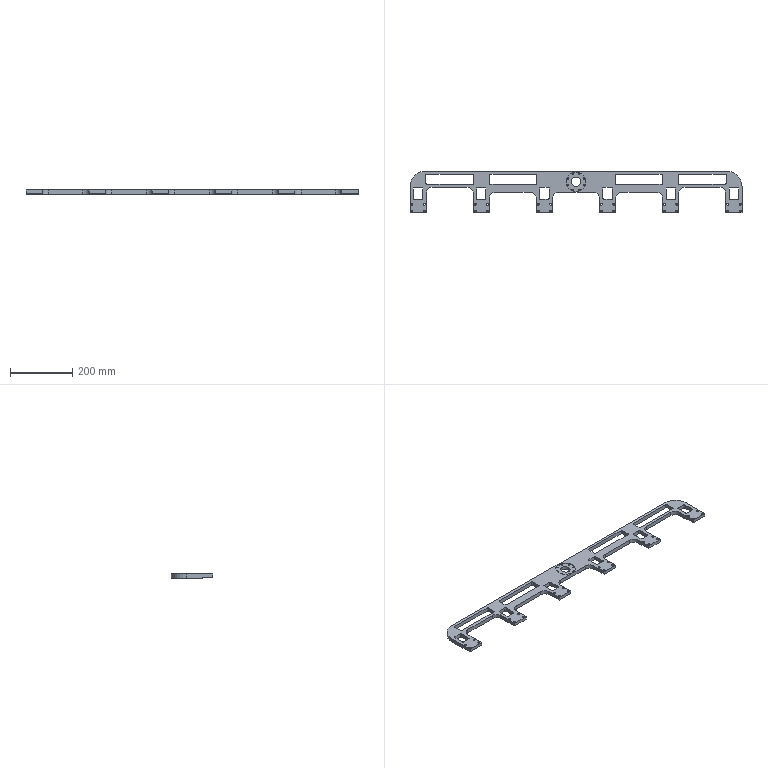NC program | NX | posted with a generic post | part box 1068 x 134 x 13 mm
Lines 9073 to 9724 of 9724:
(PLANAR_MILL_COPY_1 , TOOL : D6A45)
N18084 T07 M6
N18086 G54
N18088 G17 G0 G90 X128.785 Y-35.086 S9500 M3
N18090 G43 Z30. H7
N18092 Z0.
N18094 G94 G1 Z-1. F1400.
N18096 X128.512 Y-34.706
N18098 G3 X127.6 Y-34.295 R1.
N18100 G1 X127.5 Y-34.3
N18102 X75.7
N18104 G2 X74.7 Y-33.3 R1.
N18106 G1 Y-20.95
N18108 G3 X55.6 Y-1.85 R19.1
N18110 G1 X-55.6
N18112 G3 X-74.7 Y-20.95 R19.1
N18114 G1 Y-33.3
N18116 G2 X-75.7 Y-34.3 R1.
N18118 G1 X-127.5
N18120 G2 X-128.5 Y-33.3 R1.
N18122 G1 Y-20.95
N18124 G3 X-147.6 Y-1.85 R19.1
N18126 G1 X-258.8
N18128 G3 X-277.9 Y-20.95 R19.1
N18130 G1 Y-33.3
N18132 G2 X-278.9 Y-34.3 R1.
N18134 G1 X-330.7
N18136 G2 X-331.7 Y-33.3 R1.
N18138 G1 Y-5.
N18140 G3 X-350.8 Y14.1 R19.1
N18142 G1 X-462.
N18144 G3 X-481.1 Y-5. R19.1
N18146 G1 Y-33.3
N18148 G2 X-482.1 Y-34.3 R1.
N18150 G1 X-533.9
N18152 G2 X-534.9 Y-33.3 R1.
N18154 G1 Y17.
N18156 G2 X-484. Y67.9 R50.9
N18158 G1 X127.6
N18160 G3 X128.466 Y68.4 R1.
N18162 G1 X128.87 Y69.1
N18164 Z0.
N18166 G0 Z30.
N18168 X88.7 Y-2.73
N18170 Z0.
N18172 G1 Z-1.
N18174 X88. Y-3.134
N18176 G3 X87.5 Y-4. R1.
N18178 G1 Y-21.
N18180 G3 X89.6 Y-23.1 R2.1
N18182 G1 X113.6
N18184 G3 X115.7 Y-21. R2.1
N18186 G1 Y13.
N18188 G3 X113.6 Y15.1 R2.1
N18190 G1 X89.6
N18192 G3 X87.5 Y13. R2.1
N18194 G1 Y-4.
N18196 G3 X88. Y-4.866 R1.
N18198 G1 X88.7 Y-5.27
N18200 Z0.
N18202 G0 Z30.
N18204 X128.977 Y54.649
N18206 Z0.
N18208 G1 Z-1.
N18210 X128.34 Y55.313
N18212 G3 X127.6 Y54.64 R1.
N18214 X127.5 Y54. R2.1
N18216 G1 Y28.
N18218 G3 X127.6 Y27.36 R2.1
N18220 X128.34 Y26.687 R1.
N18222 G1 X128.977 Y27.351
N18224 Z0.
N18226 G0 Z30.
N18228 X26.469 Y45.518
N18230 Z0.
N18232 G1 Z-1.
N18234 X26.735 Y46.315
N18236 G3 X25.869 Y46.815 R1.
N18238 X22.769 Y43.715 R3.1
N18240 X25.869 Y46.815 R-3.1
N18242 X25.003 Y46.315 R1.
N18244 G1 X25.268 Y45.518
N18246 Z0.
N18248 G0 Z30.
N18250 X11.316 Y60.671
N18252 Z0.
N18254 G1 Z-1.
N18256 X11.581 Y61.469
N18258 G3 X10.715 Y61.969 R1.
N18260 X7.615 Y58.869 R3.1
N18262 X10.715 Y61.969 R-3.1
N18264 X9.849 Y61.469 R1.
N18266 G1 X10.115 Y60.671
N18268 Z0.
N18270 G0 Z30.
N18272 X-10.115
N18274 Z0.
N18276 G1 Z-1.
N18278 X-9.849 Y61.469
N18280 G3 X-10.715 Y61.969 R1.
N18282 X-13.815 Y58.869 R3.1
N18284 X-10.715 Y61.969 R-3.1
N18286 X-11.581 Y61.469 R1.
N18288 G1 X-11.316 Y60.671
N18290 Z0.
N18292 G0 Z30.
N18294 X-25.268 Y45.518
N18296 Z0.
N18298 G1 Z-1.
N18300 X-25.003 Y46.315
N18302 G3 X-25.869 Y46.815 R1.
N18304 X-28.969 Y43.715 R3.1
N18306 X-25.869 Y46.815 R-3.1
N18308 X-26.735 Y46.315 R1.
N18310 G1 X-26.469 Y45.518
N18312 Z0.
N18314 G0 Z30.
N18316 X1.309 Y45.833
N18318 Z0.
N18320 G1 Z-1.
N18322 X0.866 Y46.6
N18324 G3 X0. Y47.1 R1.
N18326 X-14.1 Y33. R14.1
N18328 X0. Y47.1 R-14.1
N18330 X-0.866 Y46.6 R1.
N18332 G1 X-1.309 Y45.833
N18334 Z0.
N18336 G0 Z30.
N18338 X26.469 Y24.087
N18340 Z0.
N18342 G1 Z-1.
N18344 X26.735 Y24.885
N18346 G3 X25.869 Y25.385 R1.
N18348 X22.769 Y22.285 R3.1
N18350 X25.869 Y25.385 R-3.1
N18352 X25.003 Y24.885 R1.
N18354 G1 X25.268 Y24.087
N18356 Z0.
N18358 G0 Z30.
N18360 X10.115 Y5.329
N18362 Z0.
N18364 G1 Z-1.
N18366 X9.849 Y4.531
N18368 G3 X10.715 Y4.031 R1.
N18370 X13.815 Y7.131 R3.1
N18372 X10.715 Y4.031 R-3.1
N18374 X11.581 Y4.531 R1.
N18376 G1 X11.316 Y5.329
N18378 Z0.
N18380 G0 Z30.
N18382 X-11.316
N18384 Z0.
N18386 G1 Z-1.
N18388 X-11.581 Y4.531
N18390 G3 X-10.715 Y4.031 R1.
N18392 X-7.615 Y7.131 R3.1
N18394 X-10.715 Y4.031 R-3.1
N18396 X-9.849 Y4.531 R1.
N18398 G1 X-10.115 Y5.329
N18400 Z0.
N18402 G0 Z30.
N18404 X-25.268 Y24.087
N18406 Z0.
N18408 G1 Z-1.
N18410 X-25.003 Y24.885
N18412 G3 X-25.869 Y25.385 R1.
N18414 X-28.969 Y22.285 R3.1
N18416 X-25.869 Y25.385 R-3.1
N18418 X-26.735 Y24.885 R1.
N18420 G1 X-26.469 Y24.087
N18422 Z0.
N18424 G0 Z30.
N18426 X-88.7 Y-5.27
N18428 Z0.
N18430 G1 Z-1.
N18432 X-88. Y-4.866
N18434 G3 X-87.5 Y-4. R1.
N18436 G1 Y13.
N18438 G3 X-89.6 Y15.1 R2.1
N18440 G1 X-113.6
N18442 G3 X-115.7 Y13. R2.1
N18444 G1 Y-21.
N18446 G3 X-113.6 Y-23.1 R2.1
N18448 G1 X-89.6
N18450 G3 X-87.5 Y-21. R2.1
N18452 G1 Y-4.
N18454 G3 X-88. Y-3.134 R1.
N18456 G1 X-88.7 Y-2.73
N18458 Z0.
N18460 G0 Z30.
N18462 X-201.93 Y54.9
N18464 Z0.
N18466 G1 Z-1.
N18468 X-202.334 Y55.6
N18470 G3 X-203.2 Y56.1 R1.
N18472 G1 X-276.8
N18474 G3 X-278.9 Y54. R2.1
N18476 G1 Y28.
N18478 G3 X-276.8 Y25.9 R2.1
N18480 G1 X-129.6
N18482 G3 X-127.5 Y28. R2.1
N18484 G1 Y54.
N18486 G3 X-129.6 Y56.1 R2.1
N18488 G1 X-203.2
N18490 G3 X-204.066 Y55.6 R1.
N18492 G1 X-204.47 Y54.9
N18494 Z0.
N18496 G0 Z30.
N18498 X-291.9 Y-5.27
N18500 Z0.
N18502 G1 Z-1.
N18504 X-291.2 Y-4.866
N18506 G3 X-290.7 Y-4. R1.
N18508 G1 Y13.
N18510 G3 X-292.8 Y15.1 R2.1
N18512 G1 X-316.8
N18514 G3 X-318.9 Y13. R2.1
N18516 G1 Y-21.
N18518 G3 X-316.8 Y-23.1 R2.1
N18520 G1 X-292.8
N18522 G3 X-290.7 Y-21. R2.1
N18524 G1 Y-4.
N18526 G3 X-291.2 Y-3.134 R1.
N18528 G1 X-291.9 Y-2.73
N18530 Z0.
N18532 G0 Z30.
N18534 X-405.13 Y54.9
N18536 Z0.
N18538 G1 Z-1.
N18540 X-405.534 Y55.6
N18542 G3 X-406.4 Y56.1 R1.
N18544 G1 X-480.
N18546 G3 X-482.1 Y54. R2.1
N18548 G1 Y28.
N18550 G3 X-480. Y25.9 R2.1
N18552 G1 X-332.8
N18554 G3 X-330.7 Y28. R2.1
N18556 G1 Y54.
N18558 G3 X-332.8 Y56.1 R2.1
N18560 G1 X-406.4
N18562 G3 X-407.266 Y55.6 R1.
N18564 G1 X-407.67 Y54.9
N18566 Z0.
N18568 G0 Z30.
N18570 X-520.9 Y-2.73
N18572 Z0.
N18574 G1 Z-1.
N18576 X-521.6 Y-3.134
N18578 G3 X-522.1 Y-4. R1.
N18580 G1 Y-21.
N18582 G3 X-520. Y-23.1 R2.1
N18584 G1 X-496.
N18586 G3 X-493.9 Y-21. R2.1
N18588 G1 Y13.
N18590 G3 X-496. Y15.1 R2.1
N18592 G1 X-520.
N18594 G3 X-522.1 Y13. R2.1
N18596 G1 Y-4.
N18598 G3 X-521.6 Y-4.866 R1.
N18600 G1 X-520.9 Y-5.27
N18602 Z0.
N18604 G0 Z30.
(PLANAR_MILL_COPY_COPY , TOOL : D6A45)
N18606 X121.593 Y-38.1
N18608 Z-3.
N18610 G1 Z-4.
N18612 Y-37.056
N18614 G3 X121.118 Y-36.9 R0.5
N18616 X122.082 Y-36.9 R-2.35
N18618 X121.607 Y-37.056 R0.5
N18620 G1 Y-38.1
N18622 Z-3.
N18624 G0 Z30.
N18626 X121.112 Y-62.242
N18628 Z-3.
N18630 G1 Z-4.
N18632 X120.734 Y-63.05
N18634 G3 X121.6 Y-63.55 R1.
N18636 X123.95 Y-61.2 R2.35
N18638 X121.6 Y-63.55 R-2.35
N18640 X122.466 Y-63.05 R1.
N18642 G1 X122.088 Y-62.242
N18644 Z-3.
N18646 G0 Z30.
N18648 X129.913 Y-37.492
N18650 Z-3.
N18652 G1 Z-4.
N18654 X129.465 Y-37.043
N18656 G3 X128.5 Y-36.782 R1.
N18658 G1 Y-66.9
N18660 G2 X127.5 Y-67.9 R1.
N18662 G1 X75.7
N18664 G2 X74.7 Y-66.9 R1.
N18666 G1 Y-36.782
N18668 G3 X73.735 Y-37.043 R1.
N18670 G1 X73.287 Y-37.492
N18672 Z-3.
N18674 G0 Z30.
N18676 X-73.287
N18678 Z-3.
N18680 G1 Z-4.
N18682 X-73.735 Y-37.043
N18684 G3 X-74.7 Y-36.782 R1.
N18686 G1 Y-66.9
N18688 G2 X-75.7 Y-67.9 R1.
N18690 G1 X-127.5
N18692 G2 X-128.5 Y-66.9 R1.
N18694 G1 Y-36.782
N18696 G3 X-129.465 Y-37.043 R1.
N18698 G1 X-129.913 Y-37.492
N18700 Z-3.
N18702 G0 Z30.
N18704 X-276.487
N18706 Z-3.
N18708 G1 Z-4.
N18710 X-276.935 Y-37.043
N18712 G3 X-277.9 Y-36.782 R1.
N18714 G1 Y-66.9
N18716 G2 X-278.9 Y-67.9 R1.
N18718 G1 X-330.7
N18720 G2 X-331.7 Y-66.9 R1.
N18722 G1 Y-36.782
N18724 G3 X-332.665 Y-37.043 R1.
N18726 G1 X-333.113 Y-37.492
N18728 Z-3.
N18730 G0 Z30.
N18732 X-479.687
N18734 Z-3.
N18736 G1 Z-4.
N18738 X-480.135 Y-37.043
N18740 G3 X-481.1 Y-36.782 R1.
N18742 G1 Y-66.9
N18744 G2 X-482.1 Y-67.9 R1.
N18746 G1 X-533.9
N18748 G2 X-534.9 Y-66.9 R1.
N18750 G1 Y-36.782
N18752 G3 X-535.865 Y-37.043 R1.
N18754 G1 X-536.313 Y-37.492
N18756 Z-3.
N18758 G0 Z30.
N18760 X81.112 Y-62.242
N18762 Z-3.
N18764 G1 Z-4.
N18766 X80.734 Y-63.05
N18768 G3 X81.6 Y-63.55 R1.
N18770 X83.95 Y-61.2 R2.35
N18772 X81.6 Y-63.55 R-2.35
N18774 X82.466 Y-63.05 R1.
N18776 G1 X82.088 Y-62.242
N18778 Z-3.
N18780 G0 Z30.
N18782 X81.593 Y-38.1
N18784 Z-3.
N18786 G1 Z-4.
N18788 Y-37.056
N18790 G3 X81.118 Y-36.9 R0.5
N18792 X82.082 Y-36.9 R-2.35
N18794 X81.607 Y-37.056 R0.5
N18796 G1 Y-38.1
N18798 Z-3.
N18800 G0 Z30.
N18802 X-81.607
N18804 Z-3.
N18806 G1 Z-4.
N18808 Y-37.056
N18810 G3 X-82.082 Y-36.9 R0.5
N18812 X-81.118 Y-36.9 R-2.35
N18814 X-81.593 Y-37.056 R0.5
N18816 G1 Y-38.1
N18818 Z-3.
N18820 G0 Z30.
N18822 X-82.088 Y-62.242
N18824 Z-3.
N18826 G1 Z-4.
N18828 X-82.466 Y-63.05
N18830 G3 X-81.6 Y-63.55 R1.
N18832 X-79.25 Y-61.2 R2.35
N18834 X-81.6 Y-63.55 R-2.35
N18836 X-80.734 Y-63.05 R1.
N18838 G1 X-81.112 Y-62.242
N18840 Z-3.
N18842 G0 Z30.
N18844 X-122.088
N18846 Z-3.
N18848 G1 Z-4.
N18850 X-122.466 Y-63.05
N18852 G3 X-121.6 Y-63.55 R1.
N18854 X-119.25 Y-61.2 R2.35
N18856 X-121.6 Y-63.55 R-2.35
N18858 X-120.734 Y-63.05 R1.
N18860 G1 X-121.112 Y-62.242
N18862 Z-3.
N18864 G0 Z30.
N18866 X-121.607 Y-38.1
N18868 Z-3.
N18870 G1 Z-4.
N18872 Y-37.056
N18874 G3 X-122.082 Y-36.9 R0.5
N18876 X-121.118 Y-36.9 R-2.35
N18878 X-121.593 Y-37.056 R0.5
N18880 G1 Y-38.1
N18882 Z-3.
N18884 G0 Z30.
N18886 X-284.807
N18888 Z-3.
N18890 G1 Z-4.
N18892 Y-37.056
N18894 G3 X-285.282 Y-36.9 R0.5
N18896 X-284.318 Y-36.9 R-2.35
N18898 X-284.793 Y-37.056 R0.5
N18900 G1 Y-38.1
N18902 Z-3.
N18904 G0 Z30.
N18906 X-285.288 Y-62.242
N18908 Z-3.
N18910 G1 Z-4.
N18912 X-285.666 Y-63.05
N18914 G3 X-284.8 Y-63.55 R1.
N18916 X-282.45 Y-61.2 R2.35
N18918 X-284.8 Y-63.55 R-2.35
N18920 X-283.934 Y-63.05 R1.
N18922 G1 X-284.312 Y-62.242
N18924 Z-3.
N18926 G0 Z30.
N18928 X-325.288
N18930 Z-3.
N18932 G1 Z-4.
N18934 X-325.666 Y-63.05
N18936 G3 X-324.8 Y-63.55 R1.
N18938 X-322.45 Y-61.2 R2.35
N18940 X-324.8 Y-63.55 R-2.35
N18942 X-323.934 Y-63.05 R1.
N18944 G1 X-324.312 Y-62.242
N18946 Z-3.
N18948 G0 Z30.
N18950 X-324.807 Y-38.1
N18952 Z-3.
N18954 G1 Z-4.
N18956 Y-37.056
N18958 G3 X-325.282 Y-36.9 R0.5
N18960 X-324.318 Y-36.9 R-2.35
N18962 X-324.793 Y-37.056 R0.5
N18964 G1 Y-38.1
N18966 Z-3.
N18968 G0 Z30.
N18970 X-488.007
N18972 Z-3.
N18974 G1 Z-4.
N18976 Y-37.056
N18978 G3 X-488.482 Y-36.9 R0.5
N18980 X-487.518 Y-36.9 R-2.35
N18982 X-487.993 Y-37.056 R0.5
N18984 G1 Y-38.1
N18986 Z-3.
N18988 G0 Z30.
N18990 X-488.488 Y-62.242
N18992 Z-3.
N18994 G1 Z-4.
N18996 X-488.866 Y-63.05
N18998 G3 X-488. Y-63.55 R1.
N19000 X-485.65 Y-61.2 R2.35
N19002 X-488. Y-63.55 R-2.35
N19004 X-487.134 Y-63.05 R1.
N19006 G1 X-487.512 Y-62.242
N19008 Z-3.
N19010 G0 Z30.
N19012 X-528.488
N19014 Z-3.
N19016 G1 Z-4.
N19018 X-528.866 Y-63.05
N19020 G3 X-528. Y-63.55 R1.
N19022 X-525.65 Y-61.2 R2.35
N19024 X-528. Y-63.55 R-2.35
N19026 X-527.134 Y-63.05 R1.
N19028 G1 X-527.512 Y-62.242
N19030 Z-3.
N19032 G0 Z30.
N19034 X-528.007 Y-38.1
N19036 Z-3.
N19038 G1 Z-4.
N19040 Y-37.056
N19042 G3 X-528.482 Y-36.9 R0.5
N19044 X-527.518 Y-36.9 R-2.35
N19046 X-527.993 Y-37.056 R0.5
N19048 G1 Y-38.1
N19050 Z-3.
N19052 G0 Z30.
N19054 M5
(ZLEVEL_PROFILE_COPY_3_COPY , TOOL : D10)
N19056 T10 M6
N19058 G54
N19060 G17 G0 G90 X129.999 Y-75.155 S9500 M3
N19062 G43 Z30. H10
N19064 Z-7.525
N19066 G94 G1 Z-12.525 F1000.
N19068 X128.466 Y-72.5
N19070 G3 X127.6 Y-72. R1.
N19072 G1 X75.6 F1200.
N19074 G2 X70.6 Y-67. R5.
N19076 G1 Y-20.95
N19078 G3 X55.6 Y-5.95 R15.
N19080 G1 X-55.6
N19082 G3 X-70.6 Y-20.95 R15.
N19084 G1 Y-67.
N19086 G2 X-75.6 Y-72. R5.
N19088 G1 X-127.6
N19090 G2 X-132.6 Y-67. R5.
N19092 G1 Y-20.95
N19094 G3 X-147.6 Y-5.95 R15.
N19096 G1 X-258.8
N19098 G3 X-273.8 Y-20.95 R15.
N19100 G1 Y-67.
N19102 G2 X-278.8 Y-72. R5.
N19104 G1 X-330.8
N19106 G2 X-335.8 Y-67. R5.
N19108 G1 Y-5.
N19110 G3 X-350.8 Y10. R15.
N19112 G1 X-462.
N19114 G3 X-477. Y-5. R15.
N19116 G1 Y-67.
N19118 G2 X-482. Y-72. R5.
N19120 G1 X-534.
N19122 G2 X-539. Y-67. R5.
N19124 G1 Y17.
N19126 G2 X-484. Y72. R55.
N19128 G1 X127.6
N19130 G3 X128.466 Y72.5 R1.
N19132 G1 X130.198 Y75.5
N19134 Z-7.525
N19136 G0 Z30.
N19138 X129.999 Y-75.155
N19140 Z-7.65
N19142 G1 Z-12.65 F1000.
N19144 X128.466 Y-72.5
N19146 G3 X127.6 Y-72. R1.
N19148 G1 X75.6 F1200.
N19150 G2 X70.6 Y-67. R5.
N19152 G1 Y-20.95
N19154 G3 X55.6 Y-5.95 R15.
N19156 G1 X-55.6
N19158 G3 X-70.6 Y-20.95 R15.
N19160 G1 Y-67.
N19162 G2 X-75.6 Y-72. R5.
N19164 G1 X-127.6
N19166 G2 X-132.6 Y-67. R5.
N19168 G1 Y-20.95
N19170 G3 X-147.6 Y-5.95 R15.
N19172 G1 X-258.8
N19174 G3 X-273.8 Y-20.95 R15.
N19176 G1 Y-67.
N19178 G2 X-278.8 Y-72. R5.
N19180 G1 X-330.8
N19182 G2 X-335.8 Y-67. R5.
N19184 G1 Y-5.
N19186 G3 X-350.8 Y10. R15.
N19188 G1 X-462.
N19190 G3 X-477. Y-5. R15.
N19192 G1 Y-67.
N19194 G2 X-482. Y-72. R5.
N19196 G1 X-534.
N19198 G2 X-539. Y-67. R5.
N19200 G1 Y17.
N19202 G2 X-484. Y72. R55.
N19204 G1 X127.6
N19206 G3 X128.466 Y72.5 R1.
N19208 G1 X130.198 Y75.5
N19210 Z-7.65
N19212 G0 Z30.
N19214 X129.999 Y-75.155
N19216 Z-7.775
N19218 G1 Z-12.775 F1000.
N19220 X128.466 Y-72.5
N19222 G3 X127.6 Y-72. R1.
N19224 G1 X75.6 F1200.
N19226 G2 X70.6 Y-67. R5.
N19228 G1 Y-20.95
N19230 G3 X55.6 Y-5.95 R15.
N19232 G1 X-55.6
N19234 G3 X-70.6 Y-20.95 R15.
N19236 G1 Y-67.
N19238 G2 X-75.6 Y-72. R5.
N19240 G1 X-127.6
N19242 G2 X-132.6 Y-67. R5.
N19244 G1 Y-20.95
N19246 G3 X-147.6 Y-5.95 R15.
N19248 G1 X-258.8
N19250 G3 X-273.8 Y-20.95 R15.
N19252 G1 Y-67.
N19254 G2 X-278.8 Y-72. R5.
N19256 G1 X-330.8
N19258 G2 X-335.8 Y-67. R5.
N19260 G1 Y-5.
N19262 G3 X-350.8 Y10. R15.
N19264 G1 X-462.
N19266 G3 X-477. Y-5. R15.
N19268 G1 Y-67.
N19270 G2 X-482. Y-72. R5.
N19272 G1 X-534.
N19274 G2 X-539. Y-67. R5.
N19276 G1 Y17.
N19278 G2 X-484. Y72. R55.
N19280 G1 X127.6
N19282 G3 X128.466 Y72.5 R1.
N19284 G1 X130.198 Y75.5
N19286 Z-7.775
N19288 G0 Z30.
N19290 X129.999 Y-75.155
N19292 Z-7.9
N19294 G1 Z-12.9 F1000.
N19296 X128.466 Y-72.5
N19298 G3 X127.6 Y-72. R1.
N19300 G1 X75.6 F1200.
N19302 G2 X70.6 Y-67. R5.
N19304 G1 Y-20.95
N19306 G3 X55.6 Y-5.95 R15.
N19308 G1 X-55.6
N19310 G3 X-70.6 Y-20.95 R15.
N19312 G1 Y-67.
N19314 G2 X-75.6 Y-72. R5.
N19316 G1 X-127.6
N19318 G2 X-132.6 Y-67. R5.
N19320 G1 Y-20.95
N19322 G3 X-147.6 Y-5.95 R15.
N19324 G1 X-258.8
N19326 G3 X-273.8 Y-20.95 R15.
N19328 G1 Y-67.
N19330 G2 X-278.8 Y-72. R5.
N19332 G1 X-330.8
N19334 G2 X-335.8 Y-67. R5.
N19336 G1 Y-5.
N19338 G3 X-350.8 Y10. R15.
N19340 G1 X-462.
N19342 G3 X-477. Y-5. R15.
N19344 G1 Y-67.
N19346 G2 X-482. Y-72. R5.
N19348 G1 X-534.
N19350 G2 X-539. Y-67. R5.
N19352 G1 Y17.
N19354 G2 X-484. Y72. R55.
N19356 G1 X127.6
N19358 G3 X128.466 Y72.5 R1.
N19360 G1 X130.198 Y75.5
N19362 Z-7.9
N19364 G0 Z30.
N19366 M5
N19368 M2